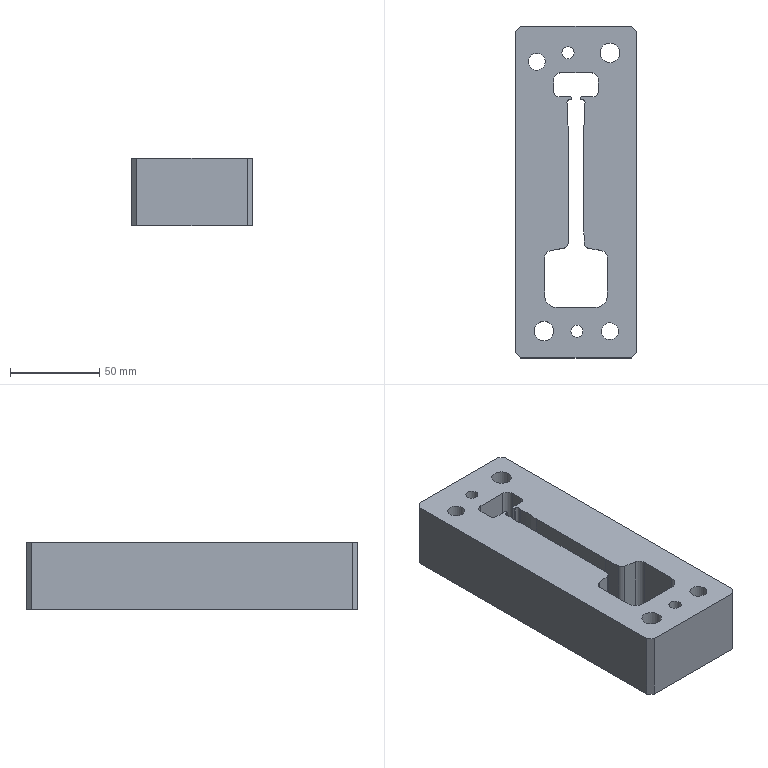Part | STEP file | 1_id202_x_t | 1 solid | 57 faces | box 68 x 186 x 38.1 mm | volume 377160 mm3 | cylinder 29 | plane 28 | commonest cylinder face diameters 1.5 x4 3 x4 6 x4 8 x4 6.8 x2 9.525 x2